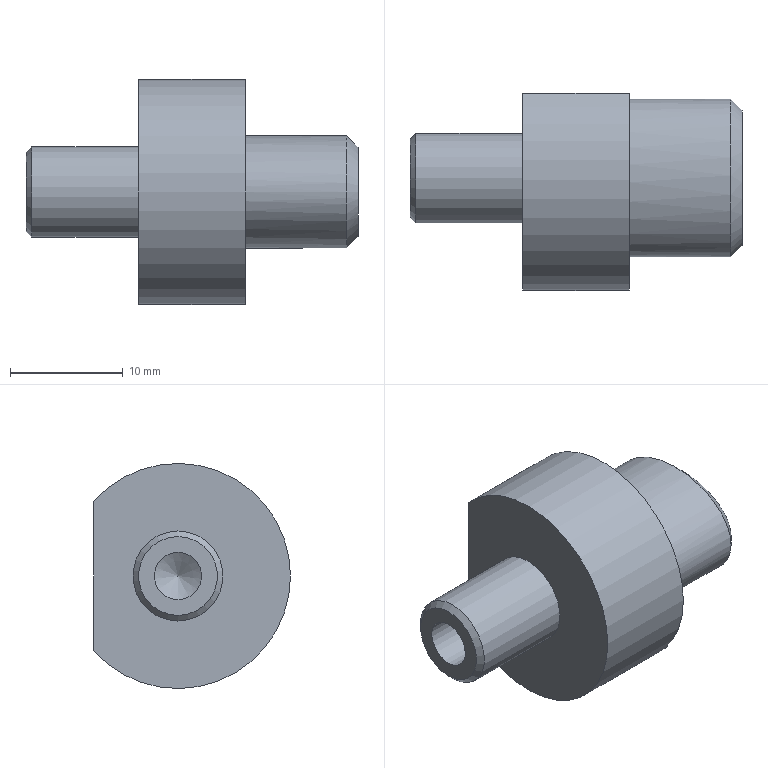Part | NX | features BREP 1 | 1 solid | 12 faces | box 29.5 x 17.5 x 20 mm | volume 4177 mm3 | plane 5 | cylinder 3 | spline 2 | cone 2 | commonest cylinder face diameters 4.2 x1 8 x1 20 x1